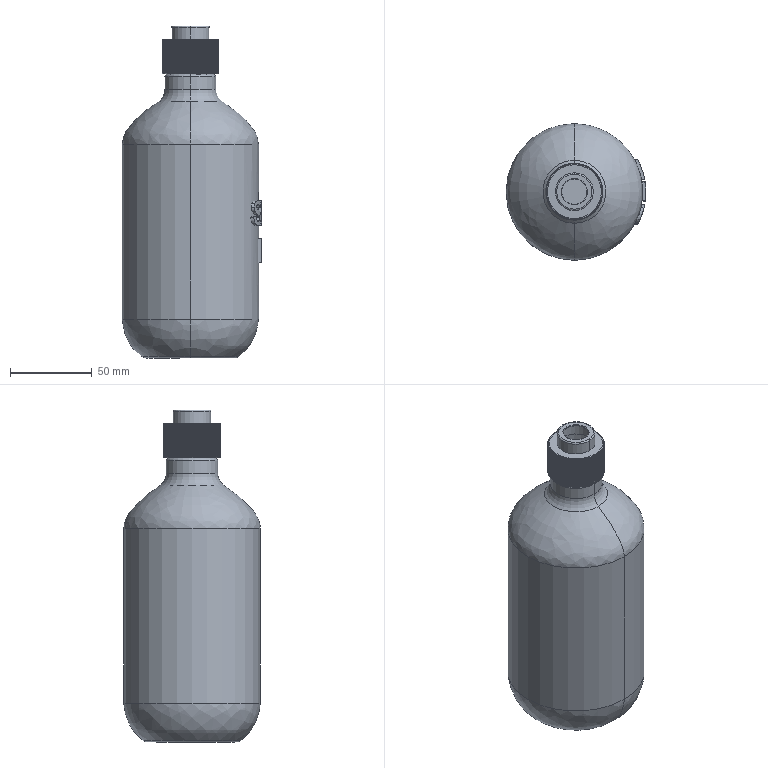Part | SolidWorks | features BaseBody 2 | 2 solids | 925 faces | box 85.56 x 83.56 x 203.378 mm | volume 49646 mm3 | cylinder 358 | spline 280 | sphere 220 | plane 39 | torus 28 | commonest cylinder face diameters 0.3 x220 0.4 x110 83.56 x8 15.567 x2 21.567 x2 23.167 x2